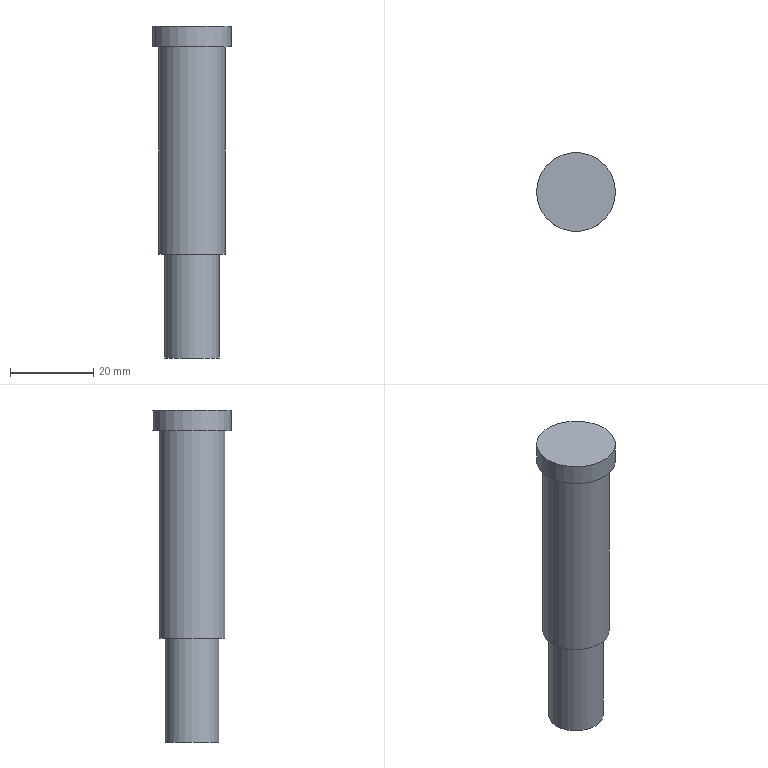Part | NX | features solid 2 | 1 solid | 7 faces | box 19 x 19 x 80 mm | volume 14840 mm3 | plane 4 | cylinder 3 | commonest cylinder face diameters 13.1 x1 16 x1 19 x1
STEP:
#1=CARTESIAN_POINT('',(-534.438,169.049,99.));
#2=VERTEX_POINT('',#1);
#3=CARTESIAN_POINT('',(-542.438,169.049,99.));
#4=DIRECTION('',(0.,0.,1.));
#5=DIRECTION('',(1.,0.,0.));
#6=AXIS2_PLACEMENT_3D('',#3,#4,#5);
#7=CIRCLE('',#6,8.);
#8=EDGE_CURVE('',#2,#2,#7,.T.);
#9=ORIENTED_EDGE('',*,*,#8,.T.);
#10=EDGE_LOOP('',(#9));
#11=FACE_BOUND('',#10,.T.);
#12=CARTESIAN_POINT('',(-534.438,169.049,149.));
#13=VERTEX_POINT('',#12);
#14=CARTESIAN_POINT('',(-542.438,169.049,149.));
#15=DIRECTION('',(0.,0.,1.));
#16=DIRECTION('',(1.,0.,0.));
#17=AXIS2_PLACEMENT_3D('',#14,#15,#16);
#18=CIRCLE('',#17,8.);
#19=EDGE_CURVE('',#13,#13,#18,.T.);
#20=ORIENTED_EDGE('',*,*,#19,.F.);
#21=EDGE_LOOP('',(#20));
#22=FACE_BOUND('',#21,.T.);
#23=CARTESIAN_POINT('',(-542.438,169.049,154.));
#24=DIRECTION('',(0.,0.,-1.));
#25=DIRECTION('',(-1.,0.,0.));
#26=AXIS2_PLACEMENT_3D('',#23,#24,#25);
#27=CYLINDRICAL_SURFACE('',#26,8.);
#28=ADVANCED_FACE('',(#11,#22),#27,.T.);
#29=CARTESIAN_POINT('',(-535.888,169.049,99.));
#30=VERTEX_POINT('',#29);
#31=CARTESIAN_POINT('',(-542.438,169.049,99.));
#32=DIRECTION('',(0.,0.,1.));
#33=DIRECTION('',(1.,0.,0.));
#34=AXIS2_PLACEMENT_3D('',#31,#32,#33);
#35=CIRCLE('',#34,6.55);
#36=EDGE_CURVE('',#30,#30,#35,.T.);
#37=ORIENTED_EDGE('',*,*,#36,.T.);
#38=EDGE_LOOP('',(#37));
#39=FACE_BOUND('',#38,.T.);
#40=ORIENTED_EDGE('',*,*,#8,.F.);
#41=EDGE_LOOP('',(#40));
#42=FACE_BOUND('',#41,.T.);
#43=CARTESIAN_POINT('',(-542.438,169.049,99.));
#44=DIRECTION('',(0.,0.,1.));
#45=DIRECTION('',(1.,0.,0.));
#46=AXIS2_PLACEMENT_3D('',#43,#44,#45);
#47=PLANE('',#46);
#48=ADVANCED_FACE('',(#39,#42),#47,.F.);
#49=CARTESIAN_POINT('',(-532.938,169.049,149.));
#50=VERTEX_POINT('',#49);
#51=CARTESIAN_POINT('',(-542.438,169.049,149.));
#52=DIRECTION('',(0.,0.,1.));
#53=DIRECTION('',(1.,0.,0.));
#54=AXIS2_PLACEMENT_3D('',#51,#52,#53);
#55=CIRCLE('',#54,9.5);
#56=EDGE_CURVE('',#50,#50,#55,.T.);
#57=ORIENTED_EDGE('',*,*,#56,.F.);
#58=EDGE_LOOP('',(#57));
#59=FACE_BOUND('',#58,.T.);
#60=ORIENTED_EDGE('',*,*,#19,.T.);
#61=EDGE_LOOP('',(#60));
#62=FACE_BOUND('',#61,.T.);
#63=CARTESIAN_POINT('',(-542.438,169.049,149.));
#64=DIRECTION('',(0.,0.,1.));
#65=DIRECTION('',(1.,0.,0.));
#66=AXIS2_PLACEMENT_3D('',#63,#64,#65);
#67=PLANE('',#66);
#68=ADVANCED_FACE('',(#59,#62),#67,.F.);
#69=ORIENTED_EDGE('',*,*,#56,.T.);
#70=EDGE_LOOP('',(#69));
#71=FACE_BOUND('',#70,.T.);
#72=CARTESIAN_POINT('',(-532.938,169.049,154.));
#73=VERTEX_POINT('',#72);
#74=CARTESIAN_POINT('',(-542.438,169.049,154.));
#75=DIRECTION('',(0.,0.,1.));
#76=DIRECTION('',(1.,0.,0.));
#77=AXIS2_PLACEMENT_3D('',#74,#75,#76);
#78=CIRCLE('',#77,9.5);
#79=EDGE_CURVE('',#73,#73,#78,.T.);
#80=ORIENTED_EDGE('',*,*,#79,.F.);
#81=EDGE_LOOP('',(#80));
#82=FACE_BOUND('',#81,.T.);
#83=CARTESIAN_POINT('',(-542.438,169.049,149.));
#84=DIRECTION('',(0.,0.,1.));
#85=DIRECTION('',(1.,0.,0.));
#86=AXIS2_PLACEMENT_3D('',#83,#84,#85);
#87=CYLINDRICAL_SURFACE('',#86,9.5);
#88=ADVANCED_FACE('',(#71,#82),#87,.T.);
#89=ORIENTED_EDGE('',*,*,#79,.T.);
#90=EDGE_LOOP('',(#89));
#91=FACE_BOUND('',#90,.T.);
#92=CARTESIAN_POINT('',(-542.438,169.049,154.));
#93=DIRECTION('',(0.,0.,1.));
#94=DIRECTION('',(1.,0.,0.));
#95=AXIS2_PLACEMENT_3D('',#92,#93,#94);
#96=PLANE('',#95);
#97=ADVANCED_FACE('',(#91),#96,.T.);
#98=CARTESIAN_POINT('',(-535.888,169.049,74.));
#99=VERTEX_POINT('',#98);
#100=CARTESIAN_POINT('',(-542.438,169.049,74.));
#101=DIRECTION('',(0.,0.,1.));
#102=DIRECTION('',(1.,0.,0.));
#103=AXIS2_PLACEMENT_3D('',#100,#101,#102);
#104=CIRCLE('',#103,6.55);
#105=EDGE_CURVE('',#99,#99,#104,.T.);
#106=ORIENTED_EDGE('',*,*,#105,.T.);
#107=EDGE_LOOP('',(#106));
#108=FACE_BOUND('',#107,.T.);
#109=ORIENTED_EDGE('',*,*,#36,.F.);
#110=EDGE_LOOP('',(#109));
#111=FACE_BOUND('',#110,.T.);
#112=CARTESIAN_POINT('',(-542.438,169.049,74.));
#113=DIRECTION('',(0.,0.,1.));
#114=DIRECTION('',(-1.,0.,0.));
#115=AXIS2_PLACEMENT_3D('',#112,#113,#114);
#116=CYLINDRICAL_SURFACE('',#115,6.55);
#117=ADVANCED_FACE('',(#108,#111),#116,.T.);
#118=ORIENTED_EDGE('',*,*,#105,.F.);
#119=EDGE_LOOP('',(#118));
#120=FACE_BOUND('',#119,.T.);
#121=CARTESIAN_POINT('',(-542.438,169.049,74.));
#122=DIRECTION('',(0.,0.,1.));
#123=DIRECTION('',(1.,0.,0.));
#124=AXIS2_PLACEMENT_3D('',#121,#122,#123);
#125=PLANE('',#124);
#126=ADVANCED_FACE('',(#120),#125,.F.);
#127=CLOSED_SHELL('',(#28,#48,#68,#88,#97,#117,#126));
#128=MANIFOLD_SOLID_BREP('',#127);
#129=(LENGTH_UNIT()NAMED_UNIT(*)SI_UNIT(.MILLI.,.METRE.));
#130=UNCERTAINTY_MEASURE_WITH_UNIT(LENGTH_MEASURE(0.00001),#129,'','');
#131=(NAMED_UNIT(*)PLANE_ANGLE_UNIT()SI_UNIT($,.RADIAN.));
#132=(NAMED_UNIT(*)SI_UNIT($,.STERADIAN.)SOLID_ANGLE_UNIT());
#133=(GEOMETRIC_REPRESENTATION_CONTEXT(3)GLOBAL_UNCERTAINTY_ASSIGNED_CONTEXT((#130))GLOBAL_UNIT_ASSIGNED_CONTEXT((#129,#131,#132))REPRESENTATION_CONTEXT('',''));
#134=ADVANCED_BREP_SHAPE_REPRESENTATION('',(#128),#133);